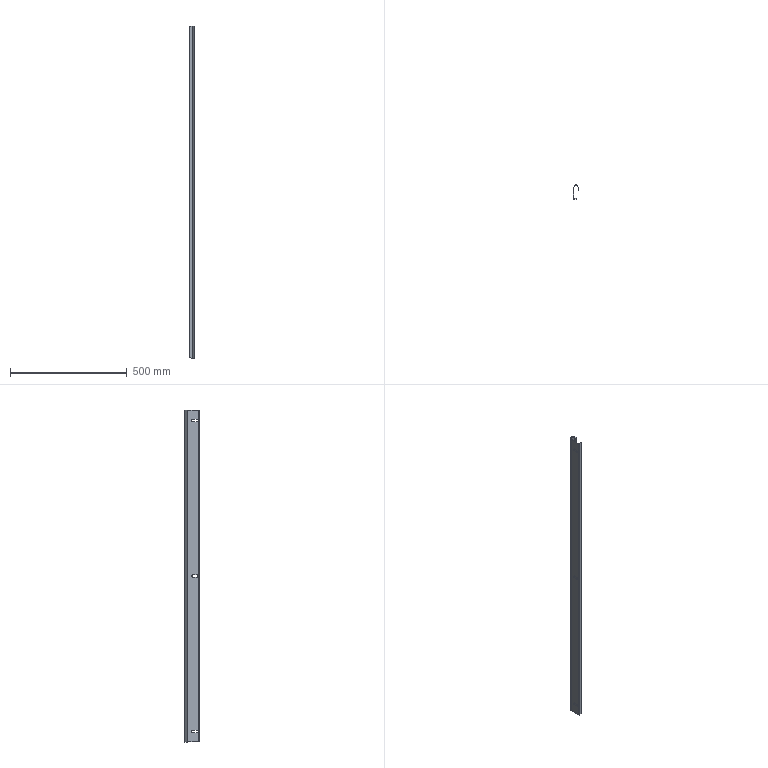Part | STEP file | Sliding Door Lower Rail | 1 solid | 34 faces | box 24 x 61.13 x 1420 mm | volume 280395 mm3 | plane 20 | cylinder 14 | commonest cylinder face diameters 9 x6 0.2 x4 4.2 x4
STEP:
#1=CARTESIAN_POINT('',(-22.,-489.271,1420.));
#2=VERTEX_POINT('',#1);
#3=CARTESIAN_POINT('',(-22.,-442.241,1420.));
#4=VERTEX_POINT('',#3);
#5=CARTESIAN_POINT('',(-22.,-441.371,1420.));
#6=DIRECTION('',(0.,1.,0.));
#7=VECTOR('',#6,1000.);
#8=LINE('',#5,#7);
#9=EDGE_CURVE('',#2,#4,#8,.T.);
#10=ORIENTED_EDGE('',*,*,#9,.T.);
#11=CARTESIAN_POINT('',(-22.,-442.241,0.));
#12=VERTEX_POINT('',#11);
#13=CARTESIAN_POINT('',(-22.,-442.241,1420.));
#14=DIRECTION('',(0.,0.,-1.));
#15=VECTOR('',#14,1000.);
#16=LINE('',#13,#15);
#17=EDGE_CURVE('',#4,#12,#16,.T.);
#18=ORIENTED_EDGE('',*,*,#17,.T.);
#19=CARTESIAN_POINT('',(-22.,-489.271,0.));
#20=VERTEX_POINT('',#19);
#21=CARTESIAN_POINT('',(-22.,-441.371,0.));
#22=DIRECTION('',(0.,-1.,0.));
#23=VECTOR('',#22,1000.);
#24=LINE('',#21,#23);
#25=EDGE_CURVE('',#12,#20,#24,.T.);
#26=ORIENTED_EDGE('',*,*,#25,.T.);
#27=CARTESIAN_POINT('',(-22.,-489.271,1420.));
#28=DIRECTION('',(0.,0.,1.));
#29=VECTOR('',#28,1000.);
#30=LINE('',#27,#29);
#31=EDGE_CURVE('',#20,#2,#30,.T.);
#32=ORIENTED_EDGE('',*,*,#31,.T.);
#33=EDGE_LOOP('',(#10,#18,#26,#32));
#34=FACE_OUTER_BOUND('',#33,.T.);
#35=CARTESIAN_POINT('',(-22.,-483.371,1379.5));
#36=VERTEX_POINT('',#35);
#37=CARTESIAN_POINT('',(-22.,-483.371,1370.5));
#38=VERTEX_POINT('',#37);
#39=CARTESIAN_POINT('',(-22.,-483.371,1375.));
#40=DIRECTION('',(1.,0.,0.));
#41=DIRECTION('',(0.,0.,-1.));
#42=AXIS2_PLACEMENT_3D('',#39,#40,#41);
#43=CIRCLE('',#42,4.5);
#44=EDGE_CURVE('',#36,#38,#43,.T.);
#45=ORIENTED_EDGE('',*,*,#44,.T.);
#46=CARTESIAN_POINT('',(-22.,-463.371,1370.5));
#47=VERTEX_POINT('',#46);
#48=CARTESIAN_POINT('',(-22.,-441.371,1370.5));
#49=DIRECTION('',(0.,1.,0.));
#50=VECTOR('',#49,1000.);
#51=LINE('',#48,#50);
#52=EDGE_CURVE('',#38,#47,#51,.T.);
#53=ORIENTED_EDGE('',*,*,#52,.T.);
#54=CARTESIAN_POINT('',(-22.,-463.371,1379.5));
#55=VERTEX_POINT('',#54);
#56=CARTESIAN_POINT('',(-22.,-463.371,1375.));
#57=DIRECTION('',(1.,0.,0.));
#58=DIRECTION('',(0.,0.,-1.));
#59=AXIS2_PLACEMENT_3D('',#56,#57,#58);
#60=CIRCLE('',#59,4.5);
#61=EDGE_CURVE('',#47,#55,#60,.T.);
#62=ORIENTED_EDGE('',*,*,#61,.T.);
#63=CARTESIAN_POINT('',(-22.,-441.371,1379.5));
#64=DIRECTION('',(0.,-1.,0.));
#65=VECTOR('',#64,1000.);
#66=LINE('',#63,#65);
#67=EDGE_CURVE('',#55,#36,#66,.T.);
#68=ORIENTED_EDGE('',*,*,#67,.T.);
#69=EDGE_LOOP('',(#45,#53,#62,#68));
#70=FACE_BOUND('',#69,.T.);
#71=CARTESIAN_POINT('',(-22.,-483.371,714.5));
#72=VERTEX_POINT('',#71);
#73=CARTESIAN_POINT('',(-22.,-483.371,705.5));
#74=VERTEX_POINT('',#73);
#75=CARTESIAN_POINT('',(-22.,-483.371,710.));
#76=DIRECTION('',(1.,0.,0.));
#77=DIRECTION('',(0.,0.,-1.));
#78=AXIS2_PLACEMENT_3D('',#75,#76,#77);
#79=CIRCLE('',#78,4.5);
#80=EDGE_CURVE('',#72,#74,#79,.T.);
#81=ORIENTED_EDGE('',*,*,#80,.T.);
#82=CARTESIAN_POINT('',(-22.,-463.371,705.5));
#83=VERTEX_POINT('',#82);
#84=CARTESIAN_POINT('',(-22.,-441.371,705.5));
#85=DIRECTION('',(0.,1.,0.));
#86=VECTOR('',#85,1000.);
#87=LINE('',#84,#86);
#88=EDGE_CURVE('',#74,#83,#87,.T.);
#89=ORIENTED_EDGE('',*,*,#88,.T.);
#90=CARTESIAN_POINT('',(-22.,-463.371,714.5));
#91=VERTEX_POINT('',#90);
#92=CARTESIAN_POINT('',(-22.,-463.371,710.));
#93=DIRECTION('',(1.,0.,0.));
#94=DIRECTION('',(0.,0.,-1.));
#95=AXIS2_PLACEMENT_3D('',#92,#93,#94);
#96=CIRCLE('',#95,4.5);
#97=EDGE_CURVE('',#83,#91,#96,.T.);
#98=ORIENTED_EDGE('',*,*,#97,.T.);
#99=CARTESIAN_POINT('',(-22.,-441.371,714.5));
#100=DIRECTION('',(0.,-1.,0.));
#101=VECTOR('',#100,1000.);
#102=LINE('',#99,#101);
#103=EDGE_CURVE('',#91,#72,#102,.T.);
#104=ORIENTED_EDGE('',*,*,#103,.T.);
#105=EDGE_LOOP('',(#81,#89,#98,#104));
#106=FACE_BOUND('',#105,.T.);
#107=CARTESIAN_POINT('',(-22.,-483.371,49.5));
#108=VERTEX_POINT('',#107);
#109=CARTESIAN_POINT('',(-22.,-483.371,40.5));
#110=VERTEX_POINT('',#109);
#111=CARTESIAN_POINT('',(-22.,-483.371,45.));
#112=DIRECTION('',(1.,0.,0.));
#113=DIRECTION('',(0.,0.,-1.));
#114=AXIS2_PLACEMENT_3D('',#111,#112,#113);
#115=CIRCLE('',#114,4.5);
#116=EDGE_CURVE('',#108,#110,#115,.T.);
#117=ORIENTED_EDGE('',*,*,#116,.T.);
#118=CARTESIAN_POINT('',(-22.,-463.371,40.5));
#119=VERTEX_POINT('',#118);
#120=CARTESIAN_POINT('',(-22.,-441.371,40.5));
#121=DIRECTION('',(0.,1.,0.));
#122=VECTOR('',#121,1000.);
#123=LINE('',#120,#122);
#124=EDGE_CURVE('',#110,#119,#123,.T.);
#125=ORIENTED_EDGE('',*,*,#124,.T.);
#126=CARTESIAN_POINT('',(-22.,-463.371,49.5));
#127=VERTEX_POINT('',#126);
#128=CARTESIAN_POINT('',(-22.,-463.371,45.));
#129=DIRECTION('',(1.,0.,0.));
#130=DIRECTION('',(0.,0.,-1.));
#131=AXIS2_PLACEMENT_3D('',#128,#129,#130);
#132=CIRCLE('',#131,4.5);
#133=EDGE_CURVE('',#119,#127,#132,.T.);
#134=ORIENTED_EDGE('',*,*,#133,.T.);
#135=CARTESIAN_POINT('',(-22.,-441.371,49.5));
#136=DIRECTION('',(0.,-1.,0.));
#137=VECTOR('',#136,1000.);
#138=LINE('',#135,#137);
#139=EDGE_CURVE('',#127,#108,#138,.T.);
#140=ORIENTED_EDGE('',*,*,#139,.T.);
#141=EDGE_LOOP('',(#117,#125,#134,#140));
#142=FACE_BOUND('',#141,.T.);
#143=CARTESIAN_POINT('',(-22.,-441.371,1420.));
#144=DIRECTION('',(-1.,0.,0.));
#145=DIRECTION('',(0.,-1.,0.));
#146=AXIS2_PLACEMENT_3D('',#143,#144,#145);
#147=PLANE('',#146);
#148=ADVANCED_FACE('',(#34,#70,#106,#142),#147,.T.);
#149=CARTESIAN_POINT('',(-21.385,-440.756,1420.));
#150=VERTEX_POINT('',#149);
#151=CARTESIAN_POINT('',(-19.9,-442.241,1420.));
#152=DIRECTION('',(0.,0.,1.));
#153=DIRECTION('',(-1.,0.,0.));
#154=AXIS2_PLACEMENT_3D('',#151,#152,#153);
#155=CIRCLE('',#154,2.1);
#156=EDGE_CURVE('',#150,#4,#155,.T.);
#157=ORIENTED_EDGE('',*,*,#156,.F.);
#158=CARTESIAN_POINT('',(-21.385,-440.756,0.));
#159=VERTEX_POINT('',#158);
#160=CARTESIAN_POINT('',(-21.385,-440.756,1420.));
#161=DIRECTION('',(0.,0.,-1.));
#162=VECTOR('',#161,1000.);
#163=LINE('',#160,#162);
#164=EDGE_CURVE('',#150,#159,#163,.T.);
#165=ORIENTED_EDGE('',*,*,#164,.T.);
#166=CARTESIAN_POINT('',(-19.9,-442.241,0.));
#167=DIRECTION('',(0.,0.,-1.));
#168=DIRECTION('',(-1.,0.,0.));
#169=AXIS2_PLACEMENT_3D('',#166,#167,#168);
#170=CIRCLE('',#169,2.1);
#171=EDGE_CURVE('',#12,#159,#170,.T.);
#172=ORIENTED_EDGE('',*,*,#171,.F.);
#173=ORIENTED_EDGE('',*,*,#17,.F.);
#174=EDGE_LOOP('',(#157,#165,#172,#173));
#175=FACE_OUTER_BOUND('',#174,.T.);
#176=CARTESIAN_POINT('',(-19.9,-442.241,1420.));
#177=DIRECTION('',(0.,0.,-1.));
#178=DIRECTION('',(-1.,0.,0.));
#179=AXIS2_PLACEMENT_3D('',#176,#177,#178);
#180=CYLINDRICAL_SURFACE('',#179,2.1);
#181=ADVANCED_FACE('',(#175),#180,.T.);
#182=CARTESIAN_POINT('',(-20.,-489.271,1420.));
#183=VERTEX_POINT('',#182);
#184=CARTESIAN_POINT('',(-20.,-442.241,1420.));
#185=VERTEX_POINT('',#184);
#186=CARTESIAN_POINT('',(-20.,-489.371,1420.));
#187=DIRECTION('',(0.,1.,0.));
#188=VECTOR('',#187,1000.);
#189=LINE('',#186,#188);
#190=EDGE_CURVE('',#183,#185,#189,.T.);
#191=ORIENTED_EDGE('',*,*,#190,.T.);
#192=CARTESIAN_POINT('',(-19.971,-442.171,1420.));
#193=VERTEX_POINT('',#192);
#194=CARTESIAN_POINT('',(-19.9,-442.241,1420.));
#195=DIRECTION('',(0.,0.,-1.));
#196=DIRECTION('',(-1.,0.,0.));
#197=AXIS2_PLACEMENT_3D('',#194,#195,#196);
#198=CIRCLE('',#197,0.1);
#199=EDGE_CURVE('',#185,#193,#198,.T.);
#200=ORIENTED_EDGE('',*,*,#199,.T.);
#201=CARTESIAN_POINT('',(-10.071,-432.271,1420.));
#202=VERTEX_POINT('',#201);
#203=CARTESIAN_POINT('',(-19.971,-442.171,1420.));
#204=DIRECTION('',(0.7071,0.7071,0.));
#205=VECTOR('',#204,1000.);
#206=LINE('',#203,#205);
#207=EDGE_CURVE('',#193,#202,#206,.T.);
#208=ORIENTED_EDGE('',*,*,#207,.T.);
#209=CARTESIAN_POINT('',(-9.929,-432.271,1420.));
#210=VERTEX_POINT('',#209);
#211=CARTESIAN_POINT('',(-10.,-432.341,1420.));
#212=DIRECTION('',(0.,0.,-1.));
#213=DIRECTION('',(-1.,0.,0.));
#214=AXIS2_PLACEMENT_3D('',#211,#212,#213);
#215=CIRCLE('',#214,0.1);
#216=EDGE_CURVE('',#202,#210,#215,.T.);
#217=ORIENTED_EDGE('',*,*,#216,.T.);
#218=CARTESIAN_POINT('',(-0.02929,-442.171,1420.));
#219=VERTEX_POINT('',#218);
#220=CARTESIAN_POINT('',(-9.929,-432.271,1420.));
#221=DIRECTION('',(0.7071,-0.7071,0.));
#222=VECTOR('',#221,1000.);
#223=LINE('',#220,#222);
#224=EDGE_CURVE('',#210,#219,#223,.T.);
#225=ORIENTED_EDGE('',*,*,#224,.T.);
#226=CARTESIAN_POINT('',(0.000000001,-442.241,1420.));
#227=VERTEX_POINT('',#226);
#228=CARTESIAN_POINT('',(-0.1,-442.241,1420.));
#229=DIRECTION('',(0.,0.,-1.));
#230=DIRECTION('',(-1.,0.,0.));
#231=AXIS2_PLACEMENT_3D('',#228,#229,#230);
#232=CIRCLE('',#231,0.1);
#233=EDGE_CURVE('',#219,#227,#232,.T.);
#234=ORIENTED_EDGE('',*,*,#233,.T.);
#235=CARTESIAN_POINT('',(0.000000001,-451.371,1420.));
#236=VERTEX_POINT('',#235);
#237=CARTESIAN_POINT('',(0.000000001,-442.171,1420.));
#238=DIRECTION('',(0.,-1.,0.));
#239=VECTOR('',#238,1000.);
#240=LINE('',#237,#239);
#241=EDGE_CURVE('',#227,#236,#240,.T.);
#242=ORIENTED_EDGE('',*,*,#241,.T.);
#243=CARTESIAN_POINT('',(2.,-451.371,1420.));
#244=VERTEX_POINT('',#243);
#245=CARTESIAN_POINT('',(2.,-451.371,1420.));
#246=DIRECTION('',(-1.,0.,0.));
#247=VECTOR('',#246,1000.);
#248=LINE('',#245,#247);
#249=EDGE_CURVE('',#244,#236,#248,.T.);
#250=ORIENTED_EDGE('',*,*,#249,.F.);
#251=CARTESIAN_POINT('',(2.,-442.241,1420.));
#252=VERTEX_POINT('',#251);
#253=CARTESIAN_POINT('',(2.,-441.371,1420.));
#254=DIRECTION('',(0.,-1.,0.));
#255=VECTOR('',#254,1000.);
#256=LINE('',#253,#255);
#257=EDGE_CURVE('',#252,#244,#256,.T.);
#258=ORIENTED_EDGE('',*,*,#257,.F.);
#259=CARTESIAN_POINT('',(1.385,-440.756,1420.));
#260=VERTEX_POINT('',#259);
#261=CARTESIAN_POINT('',(-0.1,-442.241,1420.));
#262=DIRECTION('',(0.,0.,1.));
#263=DIRECTION('',(-1.,0.,0.));
#264=AXIS2_PLACEMENT_3D('',#261,#262,#263);
#265=CIRCLE('',#264,2.1);
#266=EDGE_CURVE('',#252,#260,#265,.T.);
#267=ORIENTED_EDGE('',*,*,#266,.T.);
#268=CARTESIAN_POINT('',(-8.515,-430.856,1420.));
#269=VERTEX_POINT('',#268);
#270=CARTESIAN_POINT('',(-10.,-429.371,1420.));
#271=DIRECTION('',(0.7071,-0.7071,0.));
#272=VECTOR('',#271,1000.);
#273=LINE('',#270,#272);
#274=EDGE_CURVE('',#269,#260,#273,.T.);
#275=ORIENTED_EDGE('',*,*,#274,.F.);
#276=CARTESIAN_POINT('',(-11.485,-430.856,1420.));
#277=VERTEX_POINT('',#276);
#278=CARTESIAN_POINT('',(-10.,-432.341,1420.));
#279=DIRECTION('',(0.,0.,-1.));
#280=DIRECTION('',(-1.,0.,0.));
#281=AXIS2_PLACEMENT_3D('',#278,#279,#280);
#282=CIRCLE('',#281,2.1);
#283=EDGE_CURVE('',#277,#269,#282,.T.);
#284=ORIENTED_EDGE('',*,*,#283,.F.);
#285=CARTESIAN_POINT('',(-22.,-441.371,1420.));
#286=DIRECTION('',(0.7071,0.7071,0.));
#287=VECTOR('',#286,1000.);
#288=LINE('',#285,#287);
#289=EDGE_CURVE('',#150,#277,#288,.T.);
#290=ORIENTED_EDGE('',*,*,#289,.F.);
#291=ORIENTED_EDGE('',*,*,#156,.T.);
#292=ORIENTED_EDGE('',*,*,#9,.F.);
#293=CARTESIAN_POINT('',(-19.9,-491.371,1420.));
#294=VERTEX_POINT('',#293);
#295=CARTESIAN_POINT('',(-19.9,-489.271,1420.));
#296=DIRECTION('',(0.,0.,-1.));
#297=DIRECTION('',(-1.,0.,0.));
#298=AXIS2_PLACEMENT_3D('',#295,#296,#297);
#299=CIRCLE('',#298,2.1);
#300=EDGE_CURVE('',#294,#2,#299,.T.);
#301=ORIENTED_EDGE('',*,*,#300,.F.);
#302=CARTESIAN_POINT('',(-10.,-491.371,1420.));
#303=VERTEX_POINT('',#302);
#304=CARTESIAN_POINT('',(-22.,-491.371,1420.));
#305=DIRECTION('',(-1.,0.,0.));
#306=VECTOR('',#305,1000.);
#307=LINE('',#304,#306);
#308=EDGE_CURVE('',#303,#294,#307,.T.);
#309=ORIENTED_EDGE('',*,*,#308,.F.);
#310=CARTESIAN_POINT('',(-10.,-489.371,1420.));
#311=VERTEX_POINT('',#310);
#312=CARTESIAN_POINT('',(-10.,-442.241,1420.));
#313=DIRECTION('',(0.,1.,0.));
#314=VECTOR('',#313,1000.);
#315=LINE('',#312,#314);
#316=EDGE_CURVE('',#303,#311,#315,.T.);
#317=ORIENTED_EDGE('',*,*,#316,.T.);
#318=CARTESIAN_POINT('',(-19.9,-489.371,1420.));
#319=VERTEX_POINT('',#318);
#320=CARTESIAN_POINT('',(-0.1,-489.371,1420.));
#321=DIRECTION('',(-1.,0.,0.));
#322=VECTOR('',#321,1000.);
#323=LINE('',#320,#322);
#324=EDGE_CURVE('',#311,#319,#323,.T.);
#325=ORIENTED_EDGE('',*,*,#324,.T.);
#326=CARTESIAN_POINT('',(-19.9,-489.271,1420.));
#327=DIRECTION('',(0.,0.,-1.));
#328=DIRECTION('',(-1.,0.,0.));
#329=AXIS2_PLACEMENT_3D('',#326,#327,#328);
#330=CIRCLE('',#329,0.1);
#331=EDGE_CURVE('',#319,#183,#330,.T.);
#332=ORIENTED_EDGE('',*,*,#331,.T.);
#333=EDGE_LOOP('',(#191,#200,#208,#217,#225,#234,#242,#250,#258,#267,#275,#284,#290,#291,#292,#301,#309,#317,#325,#332));
#334=FACE_OUTER_BOUND('',#333,.T.);
#335=CARTESIAN_POINT('',(-19.9,-489.371,1420.));
#336=DIRECTION('',(0.,0.,1.));
#337=DIRECTION('',(1.,0.,0.));
#338=AXIS2_PLACEMENT_3D('',#335,#336,#337);
#339=PLANE('',#338);
#340=ADVANCED_FACE('',(#334),#339,.T.);
#341=ORIENTED_EDGE('',*,*,#300,.T.);
#342=ORIENTED_EDGE('',*,*,#31,.F.);
#343=CARTESIAN_POINT('',(-19.9,-491.371,0.));
#344=VERTEX_POINT('',#343);
#345=CARTESIAN_POINT('',(-19.9,-489.271,0.));
#346=DIRECTION('',(0.,0.,1.));
#347=DIRECTION('',(-1.,0.,0.));
#348=AXIS2_PLACEMENT_3D('',#345,#346,#347);
#349=CIRCLE('',#348,2.1);
#350=EDGE_CURVE('',#20,#344,#349,.T.);
#351=ORIENTED_EDGE('',*,*,#350,.T.);
#352=CARTESIAN_POINT('',(-19.9,-491.371,1420.));
#353=DIRECTION('',(0.,0.,1.));
#354=VECTOR('',#353,1000.);
#355=LINE('',#352,#354);
#356=EDGE_CURVE('',#344,#294,#355,.T.);
#357=ORIENTED_EDGE('',*,*,#356,.T.);
#358=EDGE_LOOP('',(#341,#342,#351,#357));
#359=FACE_OUTER_BOUND('',#358,.T.);
#360=CARTESIAN_POINT('',(-19.9,-489.271,1420.));
#361=DIRECTION('',(0.,0.,-1.));
#362=DIRECTION('',(-1.,0.,0.));
#363=AXIS2_PLACEMENT_3D('',#360,#361,#362);
#364=CYLINDRICAL_SURFACE('',#363,2.1);
#365=ADVANCED_FACE('',(#359),#364,.T.);
#366=CARTESIAN_POINT('',(-20.,-442.241,0.));
#367=VERTEX_POINT('',#366);
#368=CARTESIAN_POINT('',(-20.,-489.271,0.));
#369=VERTEX_POINT('',#368);
#370=CARTESIAN_POINT('',(-20.,-442.171,0.));
#371=DIRECTION('',(0.,-1.,0.));
#372=VECTOR('',#371,1000.);
#373=LINE('',#370,#372);
#374=EDGE_CURVE('',#367,#369,#373,.T.);
#375=ORIENTED_EDGE('',*,*,#374,.T.);
#376=CARTESIAN_POINT('',(-19.9,-489.371,0.));
#377=VERTEX_POINT('',#376);
#378=CARTESIAN_POINT('',(-19.9,-489.271,0.));
#379=DIRECTION('',(0.,0.,1.));
#380=DIRECTION('',(-1.,0.,0.));
#381=AXIS2_PLACEMENT_3D('',#378,#379,#380);
#382=CIRCLE('',#381,0.1);
#383=EDGE_CURVE('',#369,#377,#382,.T.);
#384=ORIENTED_EDGE('',*,*,#383,.T.);
#385=CARTESIAN_POINT('',(-10.,-489.371,0.));
#386=VERTEX_POINT('',#385);
#387=CARTESIAN_POINT('',(-20.,-489.371,0.));
#388=DIRECTION('',(1.,0.,0.));
#389=VECTOR('',#388,1000.);
#390=LINE('',#387,#389);
#391=EDGE_CURVE('',#377,#386,#390,.T.);
#392=ORIENTED_EDGE('',*,*,#391,.T.);
#393=CARTESIAN_POINT('',(-10.,-491.371,0.));
#394=VERTEX_POINT('',#393);
#395=CARTESIAN_POINT('',(-10.,-489.371,0.));
#396=DIRECTION('',(0.,1.,0.));
#397=VECTOR('',#396,1000.);
#398=LINE('',#395,#397);
#399=EDGE_CURVE('',#394,#386,#398,.T.);
#400=ORIENTED_EDGE('',*,*,#399,.F.);
#401=CARTESIAN_POINT('',(-22.,-491.371,0.));
#402=DIRECTION('',(1.,0.,0.));
#403=VECTOR('',#402,1000.);
#404=LINE('',#401,#403);
#405=EDGE_CURVE('',#344,#394,#404,.T.);
#406=ORIENTED_EDGE('',*,*,#405,.F.);
#407=ORIENTED_EDGE('',*,*,#350,.F.);
#408=ORIENTED_EDGE('',*,*,#25,.F.);
#409=ORIENTED_EDGE('',*,*,#171,.T.);
#410=CARTESIAN_POINT('',(-11.485,-430.856,0.));
#411=VERTEX_POINT('',#410);
#412=CARTESIAN_POINT('',(-22.,-441.371,0.));
#413=DIRECTION('',(-0.7071,-0.7071,0.));
#414=VECTOR('',#413,1000.);
#415=LINE('',#412,#414);
#416=EDGE_CURVE('',#411,#159,#415,.T.);
#417=ORIENTED_EDGE('',*,*,#416,.F.);
#418=CARTESIAN_POINT('',(-8.515,-430.856,0.));
#419=VERTEX_POINT('',#418);
#420=CARTESIAN_POINT('',(-10.,-432.341,0.));
#421=DIRECTION('',(0.,0.,1.));
#422=DIRECTION('',(-1.,0.,0.));
#423=AXIS2_PLACEMENT_3D('',#420,#421,#422);
#424=CIRCLE('',#423,2.1);
#425=EDGE_CURVE('',#419,#411,#424,.T.);
#426=ORIENTED_EDGE('',*,*,#425,.F.);
#427=CARTESIAN_POINT('',(1.385,-440.756,0.));
#428=VERTEX_POINT('',#427);
#429=CARTESIAN_POINT('',(-10.,-429.371,0.));
#430=DIRECTION('',(-0.7071,0.7071,0.));
#431=VECTOR('',#430,1000.);
#432=LINE('',#429,#431);
#433=EDGE_CURVE('',#428,#419,#432,.T.);
#434=ORIENTED_EDGE('',*,*,#433,.F.);
#435=CARTESIAN_POINT('',(2.,-442.241,0.));
#436=VERTEX_POINT('',#435);
#437=CARTESIAN_POINT('',(-0.1,-442.241,0.));
#438=DIRECTION('',(0.,0.,-1.));
#439=DIRECTION('',(-1.,0.,0.));
#440=AXIS2_PLACEMENT_3D('',#437,#438,#439);
#441=CIRCLE('',#440,2.1);
#442=EDGE_CURVE('',#428,#436,#441,.T.);
#443=ORIENTED_EDGE('',*,*,#442,.T.);
#444=CARTESIAN_POINT('',(2.,-451.371,0.));
#445=VERTEX_POINT('',#444);
#446=CARTESIAN_POINT('',(2.,-441.371,0.));
#447=DIRECTION('',(0.,1.,0.));
#448=VECTOR('',#447,1000.);
#449=LINE('',#446,#448);
#450=EDGE_CURVE('',#445,#436,#449,.T.);
#451=ORIENTED_EDGE('',*,*,#450,.F.);
#452=CARTESIAN_POINT('',(0.000000001,-451.371,0.));
#453=VERTEX_POINT('',#452);
#454=CARTESIAN_POINT('',(2.,-451.371,0.));
#455=DIRECTION('',(1.,0.,0.));
#456=VECTOR('',#455,1000.);
#457=LINE('',#454,#456);
#458=EDGE_CURVE('',#453,#445,#457,.T.);
#459=ORIENTED_EDGE('',*,*,#458,.F.);
#460=CARTESIAN_POINT('',(0.000000001,-442.241,0.));
#461=VERTEX_POINT('',#460);
#462=CARTESIAN_POINT('',(0.000000001,-442.241,0.));
#463=DIRECTION('',(0.,-1.,0.));
#464=VECTOR('',#463,1000.);
#465=LINE('',#462,#464);
#466=EDGE_CURVE('',#461,#453,#465,.T.);
#467=ORIENTED_EDGE('',*,*,#466,.F.);
#468=CARTESIAN_POINT('',(-0.02929,-442.171,0.));
#469=VERTEX_POINT('',#468);
#470=CARTESIAN_POINT('',(-0.1,-442.241,0.));
#471=DIRECTION('',(0.,0.,1.));
#472=DIRECTION('',(-1.,0.,0.));
#473=AXIS2_PLACEMENT_3D('',#470,#471,#472);
#474=CIRCLE('',#473,0.1);
#475=EDGE_CURVE('',#461,#469,#474,.T.);
#476=ORIENTED_EDGE('',*,*,#475,.T.);
#477=CARTESIAN_POINT('',(-9.929,-432.271,0.));
#478=VERTEX_POINT('',#477);
#479=CARTESIAN_POINT('',(-0.02929,-442.171,0.));
#480=DIRECTION('',(-0.7071,0.7071,0.));
#481=VECTOR('',#480,1000.);
#482=LINE('',#479,#481);
#483=EDGE_CURVE('',#469,#478,#482,.T.);
#484=ORIENTED_EDGE('',*,*,#483,.T.);
#485=CARTESIAN_POINT('',(-10.071,-432.271,0.));
#486=VERTEX_POINT('',#485);
#487=CARTESIAN_POINT('',(-10.,-432.341,0.));
#488=DIRECTION('',(0.,0.,1.));
#489=DIRECTION('',(-1.,0.,0.));
#490=AXIS2_PLACEMENT_3D('',#487,#488,#489);
#491=CIRCLE('',#490,0.1);
#492=EDGE_CURVE('',#478,#486,#491,.T.);
#493=ORIENTED_EDGE('',*,*,#492,.T.);
#494=CARTESIAN_POINT('',(-19.971,-442.171,0.));
#495=VERTEX_POINT('',#494);
#496=CARTESIAN_POINT('',(-10.071,-432.271,0.));
#497=DIRECTION('',(-0.7071,-0.7071,0.));
#498=VECTOR('',#497,1000.);
#499=LINE('',#496,#498);
#500=EDGE_CURVE('',#486,#495,#499,.T.);
#501=ORIENTED_EDGE('',*,*,#500,.T.);
#502=CARTESIAN_POINT('',(-19.9,-442.241,0.));
#503=DIRECTION('',(0.,0.,1.));
#504=DIRECTION('',(-1.,0.,0.));
#505=AXIS2_PLACEMENT_3D('',#502,#503,#504);
#506=CIRCLE('',#505,0.1);
#507=EDGE_CURVE('',#495,#367,#506,.T.);
#508=ORIENTED_EDGE('',*,*,#507,.T.);
#509=EDGE_LOOP('',(#375,#384,#392,#400,#406,#407,#408,#409,#417,#426,#434,#443,#451,#459,#467,#476,#484,#493,#501,#508));
#510=FACE_OUTER_BOUND('',#509,.T.);
#511=CARTESIAN_POINT('',(-19.971,-442.171,0.));
#512=DIRECTION('',(0.,0.,-1.));
#513=DIRECTION('',(-1.,0.,0.));
#514=AXIS2_PLACEMENT_3D('',#511,#512,#513);
#515=PLANE('',#514);
#516=ADVANCED_FACE('',(#510),#515,.T.);
#517=CARTESIAN_POINT('',(-20.,-483.371,1370.5));
#518=VERTEX_POINT('',#517);
#519=CARTESIAN_POINT('',(-30.,-483.371,1370.5));
#520=DIRECTION('',(-1.,0.,0.));
#521=VECTOR('',#520,1000.);
#522=LINE('',#519,#521);
#523=EDGE_CURVE('',#518,#38,#522,.T.);
#524=ORIENTED_EDGE('',*,*,#523,.F.);
#525=CARTESIAN_POINT('',(-20.,-463.371,1370.5));
#526=VERTEX_POINT('',#525);
#527=CARTESIAN_POINT('',(-20.,-463.371,1370.5));
#528=DIRECTION('',(0.,-1.,0.));
#529=VECTOR('',#528,1000.);
#530=LINE('',#527,#529);
#531=EDGE_CURVE('',#526,#518,#530,.T.);
#532=ORIENTED_EDGE('',*,*,#531,.F.);
#533=CARTESIAN_POINT('',(-30.,-463.371,1370.5));
#534=DIRECTION('',(1.,0.,0.));
#535=VECTOR('',#534,1000.);
#536=LINE('',#533,#535);
#537=EDGE_CURVE('',#47,#526,#536,.T.);
#538=ORIENTED_EDGE('',*,*,#537,.F.);
#539=ORIENTED_EDGE('',*,*,#52,.F.);
#540=EDGE_LOOP('',(#524,#532,#538,#539));
#541=FACE_OUTER_BOUND('',#540,.T.);
#542=CARTESIAN_POINT('',(-30.,-463.371,1370.5));
#543=DIRECTION('',(0.,0.,-1.));
#544=DIRECTION('',(-1.,0.,0.));
#545=AXIS2_PLACEMENT_3D('',#542,#543,#544);
#546=PLANE('',#545);
#547=ADVANCED_FACE('',(#541),#546,.F.);
#548=CARTESIAN_POINT('',(-20.,-483.371,1379.5));
#549=VERTEX_POINT('',#548);
#550=CARTESIAN_POINT('',(-30.,-483.371,1379.5));
#551=DIRECTION('',(-1.,0.,0.));
#552=VECTOR('',#551,1000.);
#553=LINE('',#550,#552);
#554=EDGE_CURVE('',#549,#36,#553,.T.);
#555=ORIENTED_EDGE('',*,*,#554,.F.);
#556=CARTESIAN_POINT('',(-20.,-483.371,1375.));
#557=DIRECTION('',(-1.,0.,0.));
#558=DIRECTION('',(0.,0.,-1.));
#559=AXIS2_PLACEMENT_3D('',#556,#557,#558);
#560=CIRCLE('',#559,4.5);
#561=EDGE_CURVE('',#518,#549,#560,.T.);
#562=ORIENTED_EDGE('',*,*,#561,.F.);
#563=ORIENTED_EDGE('',*,*,#523,.T.);
#564=ORIENTED_EDGE('',*,*,#44,.F.);
#565=EDGE_LOOP('',(#555,#562,#563,#564));
#566=FACE_OUTER_BOUND('',#565,.T.);
#567=CARTESIAN_POINT('',(-30.,-483.371,1375.));
#568=DIRECTION('',(1.,0.,0.));
#569=DIRECTION('',(0.,0.,-1.));
#570=AXIS2_PLACEMENT_3D('',#567,#568,#569);
#571=CYLINDRICAL_SURFACE('',#570,4.5);
#572=ADVANCED_FACE('',(#566),#571,.F.);
#573=CARTESIAN_POINT('',(-20.,-463.371,1379.5));
#574=VERTEX_POINT('',#573);
#575=CARTESIAN_POINT('',(-30.,-463.371,1379.5));
#576=DIRECTION('',(-1.,0.,0.));
#577=VECTOR('',#576,1000.);
#578=LINE('',#575,#577);
#579=EDGE_CURVE('',#574,#55,#578,.T.);
#580=ORIENTED_EDGE('',*,*,#579,.F.);
#581=CARTESIAN_POINT('',(-20.,-463.371,1379.5));
#582=DIRECTION('',(0.,1.,0.));
#583=VECTOR('',#582,1000.);
#584=LINE('',#581,#583);
#585=EDGE_CURVE('',#549,#574,#584,.T.);
#586=ORIENTED_EDGE('',*,*,#585,.F.);
#587=ORIENTED_EDGE('',*,*,#554,.T.);
#588=ORIENTED_EDGE('',*,*,#67,.F.);
#589=EDGE_LOOP('',(#580,#586,#587,#588));
#590=FACE_OUTER_BOUND('',#589,.T.);
#591=CARTESIAN_POINT('',(-30.,-463.371,1379.5));
#592=DIRECTION('',(0.,0.,1.));
#593=DIRECTION('',(1.,0.,0.));
#594=AXIS2_PLACEMENT_3D('',#591,#592,#593);
#595=PLANE('',#594);
#596=ADVANCED_FACE('',(#590),#595,.F.);
#597=ORIENTED_EDGE('',*,*,#537,.T.);
#598=CARTESIAN_POINT('',(-20.,-463.371,1375.));
#599=DIRECTION('',(-1.,0.,0.));
#600=DIRECTION('',(0.,0.,-1.));
#601=AXIS2_PLACEMENT_3D('',#598,#599,#600);
#602=CIRCLE('',#601,4.5);
#603=EDGE_CURVE('',#574,#526,#602,.T.);
#604=ORIENTED_EDGE('',*,*,#603,.F.);
#605=ORIENTED_EDGE('',*,*,#579,.T.);
#606=ORIENTED_EDGE('',*,*,#61,.F.);
#607=EDGE_LOOP('',(#597,#604,#605,#606));
#608=FACE_OUTER_BOUND('',#607,.T.);
#609=CARTESIAN_POINT('',(-30.,-463.371,1375.));
#610=DIRECTION('',(1.,0.,0.));
#611=DIRECTION('',(0.,0.,-1.));
#612=AXIS2_PLACEMENT_3D('',#609,#610,#611);
#613=CYLINDRICAL_SURFACE('',#612,4.5);
#614=ADVANCED_FACE('',(#608),#613,.F.);
#615=CARTESIAN_POINT('',(-20.,-483.371,705.5));
#616=VERTEX_POINT('',#615);
#617=CARTESIAN_POINT('',(-30.,-483.371,705.5));
#618=DIRECTION('',(-1.,0.,0.));
#619=VECTOR('',#618,1000.);
#620=LINE('',#617,#619);
#621=EDGE_CURVE('',#616,#74,#620,.T.);
#622=ORIENTED_EDGE('',*,*,#621,.F.);
#623=CARTESIAN_POINT('',(-20.,-463.371,705.5));
#624=VERTEX_POINT('',#623);
#625=CARTESIAN_POINT('',(-20.,-463.371,705.5));
#626=DIRECTION('',(0.,-1.,0.));
#627=VECTOR('',#626,1000.);
#628=LINE('',#625,#627);
#629=EDGE_CURVE('',#624,#616,#628,.T.);
#630=ORIENTED_EDGE('',*,*,#629,.F.);
#631=CARTESIAN_POINT('',(-30.,-463.371,705.5));
#632=DIRECTION('',(1.,0.,0.));
#633=VECTOR('',#632,1000.);
#634=LINE('',#631,#633);
#635=EDGE_CURVE('',#83,#624,#634,.T.);
#636=ORIENTED_EDGE('',*,*,#635,.F.);
#637=ORIENTED_EDGE('',*,*,#88,.F.);
#638=EDGE_LOOP('',(#622,#630,#636,#637));
#639=FACE_OUTER_BOUND('',#638,.T.);
#640=CARTESIAN_POINT('',(-30.,-463.371,705.5));
#641=DIRECTION('',(0.,0.,-1.));
#642=DIRECTION('',(-1.,0.,0.));
#643=AXIS2_PLACEMENT_3D('',#640,#641,#642);
#644=PLANE('',#643);
#645=ADVANCED_FACE('',(#639),#644,.F.);
#646=CARTESIAN_POINT('',(-20.,-483.371,714.5));
#647=VERTEX_POINT('',#646);
#648=CARTESIAN_POINT('',(-30.,-483.371,714.5));
#649=DIRECTION('',(-1.,0.,0.));
#650=VECTOR('',#649,1000.);
#651=LINE('',#648,#650);
#652=EDGE_CURVE('',#647,#72,#651,.T.);
#653=ORIENTED_EDGE('',*,*,#652,.F.);
#654=CARTESIAN_POINT('',(-20.,-483.371,710.));
#655=DIRECTION('',(-1.,0.,0.));
#656=DIRECTION('',(0.,0.,-1.));
#657=AXIS2_PLACEMENT_3D('',#654,#655,#656);
#658=CIRCLE('',#657,4.5);
#659=EDGE_CURVE('',#616,#647,#658,.T.);
#660=ORIENTED_EDGE('',*,*,#659,.F.);
#661=ORIENTED_EDGE('',*,*,#621,.T.);
#662=ORIENTED_EDGE('',*,*,#80,.F.);
#663=EDGE_LOOP('',(#653,#660,#661,#662));
#664=FACE_OUTER_BOUND('',#663,.T.);
#665=CARTESIAN_POINT('',(-30.,-483.371,710.));
#666=DIRECTION('',(1.,0.,0.));
#667=DIRECTION('',(0.,0.,-1.));
#668=AXIS2_PLACEMENT_3D('',#665,#666,#667);
#669=CYLINDRICAL_SURFACE('',#668,4.5);
#670=ADVANCED_FACE('',(#664),#669,.F.);
#671=CARTESIAN_POINT('',(-20.,-463.371,714.5));
#672=VERTEX_POINT('',#671);
#673=CARTESIAN_POINT('',(-30.,-463.371,714.5));
#674=DIRECTION('',(-1.,0.,0.));
#675=VECTOR('',#674,1000.);
#676=LINE('',#673,#675);
#677=EDGE_CURVE('',#672,#91,#676,.T.);
#678=ORIENTED_EDGE('',*,*,#677,.F.);
#679=CARTESIAN_POINT('',(-20.,-463.371,714.5));
#680=DIRECTION('',(0.,1.,0.));
#681=VECTOR('',#680,1000.);
#682=LINE('',#679,#681);
#683=EDGE_CURVE('',#647,#672,#682,.T.);
#684=ORIENTED_EDGE('',*,*,#683,.F.);
#685=ORIENTED_EDGE('',*,*,#652,.T.);
#686=ORIENTED_EDGE('',*,*,#103,.F.);
#687=EDGE_LOOP('',(#678,#684,#685,#686));
#688=FACE_OUTER_BOUND('',#687,.T.);
#689=CARTESIAN_POINT('',(-30.,-463.371,714.5));
#690=DIRECTION('',(0.,0.,1.));
#691=DIRECTION('',(1.,0.,0.));
#692=AXIS2_PLACEMENT_3D('',#689,#690,#691);
#693=PLANE('',#692);
#694=ADVANCED_FACE('',(#688),#693,.F.);
#695=ORIENTED_EDGE('',*,*,#635,.T.);
#696=CARTESIAN_POINT('',(-20.,-463.371,710.));
#697=DIRECTION('',(-1.,0.,0.));
#698=DIRECTION('',(0.,0.,-1.));
#699=AXIS2_PLACEMENT_3D('',#696,#697,#698);
#700=CIRCLE('',#699,4.5);
#701=EDGE_CURVE('',#672,#624,#700,.T.);
#702=ORIENTED_EDGE('',*,*,#701,.F.);
#703=ORIENTED_EDGE('',*,*,#677,.T.);
#704=ORIENTED_EDGE('',*,*,#97,.F.);
#705=EDGE_LOOP('',(#695,#702,#703,#704));
#706=FACE_OUTER_BOUND('',#705,.T.);
#707=CARTESIAN_POINT('',(-30.,-463.371,710.));
#708=DIRECTION('',(1.,0.,0.));
#709=DIRECTION('',(0.,0.,-1.));
#710=AXIS2_PLACEMENT_3D('',#707,#708,#709);
#711=CYLINDRICAL_SURFACE('',#710,4.5);
#712=ADVANCED_FACE('',(#706),#711,.F.);
#713=CARTESIAN_POINT('',(-20.,-483.371,40.5));
#714=VERTEX_POINT('',#713);
#715=CARTESIAN_POINT('',(-30.,-483.371,40.5));
#716=DIRECTION('',(-1.,0.,0.));
#717=VECTOR('',#716,1000.);
#718=LINE('',#715,#717);
#719=EDGE_CURVE('',#714,#110,#718,.T.);
#720=ORIENTED_EDGE('',*,*,#719,.F.);
#721=CARTESIAN_POINT('',(-20.,-463.371,40.5));
#722=VERTEX_POINT('',#721);
#723=CARTESIAN_POINT('',(-20.,-463.371,40.5));
#724=DIRECTION('',(0.,-1.,0.));
#725=VECTOR('',#724,1000.);
#726=LINE('',#723,#725);
#727=EDGE_CURVE('',#722,#714,#726,.T.);
#728=ORIENTED_EDGE('',*,*,#727,.F.);
#729=CARTESIAN_POINT('',(-30.,-463.371,40.5));
#730=DIRECTION('',(1.,0.,0.));
#731=VECTOR('',#730,1000.);
#732=LINE('',#729,#731);
#733=EDGE_CURVE('',#119,#722,#732,.T.);
#734=ORIENTED_EDGE('',*,*,#733,.F.);
#735=ORIENTED_EDGE('',*,*,#124,.F.);
#736=EDGE_LOOP('',(#720,#728,#734,#735));
#737=FACE_OUTER_BOUND('',#736,.T.);
#738=CARTESIAN_POINT('',(-30.,-463.371,40.5));
#739=DIRECTION('',(0.,0.,-1.));
#740=DIRECTION('',(-1.,0.,0.));
#741=AXIS2_PLACEMENT_3D('',#738,#739,#740);
#742=PLANE('',#741);
#743=ADVANCED_FACE('',(#737),#742,.F.);
#744=CARTESIAN_POINT('',(-20.,-483.371,49.5));
#745=VERTEX_POINT('',#744);
#746=CARTESIAN_POINT('',(-30.,-483.371,49.5));
#747=DIRECTION('',(-1.,0.,0.));
#748=VECTOR('',#747,1000.);
#749=LINE('',#746,#748);
#750=EDGE_CURVE('',#745,#108,#749,.T.);
#751=ORIENTED_EDGE('',*,*,#750,.F.);
#752=CARTESIAN_POINT('',(-20.,-483.371,45.));
#753=DIRECTION('',(-1.,0.,0.));
#754=DIRECTION('',(0.,0.,-1.));
#755=AXIS2_PLACEMENT_3D('',#752,#753,#754);
#756=CIRCLE('',#755,4.5);
#757=EDGE_CURVE('',#714,#745,#756,.T.);
#758=ORIENTED_EDGE('',*,*,#757,.F.);
#759=ORIENTED_EDGE('',*,*,#719,.T.);
#760=ORIENTED_EDGE('',*,*,#116,.F.);
#761=EDGE_LOOP('',(#751,#758,#759,#760));
#762=FACE_OUTER_BOUND('',#761,.T.);
#763=CARTESIAN_POINT('',(-30.,-483.371,45.));
#764=DIRECTION('',(1.,0.,0.));
#765=DIRECTION('',(0.,0.,-1.));
#766=AXIS2_PLACEMENT_3D('',#763,#764,#765);
#767=CYLINDRICAL_SURFACE('',#766,4.5);
#768=ADVANCED_FACE('',(#762),#767,.F.);
#769=CARTESIAN_POINT('',(-20.,-463.371,49.5));
#770=VERTEX_POINT('',#769);
#771=CARTESIAN_POINT('',(-30.,-463.371,49.5));
#772=DIRECTION('',(-1.,0.,0.));
#773=VECTOR('',#772,1000.);
#774=LINE('',#771,#773);
#775=EDGE_CURVE('',#770,#127,#774,.T.);
#776=ORIENTED_EDGE('',*,*,#775,.F.);
#777=CARTESIAN_POINT('',(-20.,-463.371,49.5));
#778=DIRECTION('',(0.,1.,0.));
#779=VECTOR('',#778,1000.);
#780=LINE('',#777,#779);
#781=EDGE_CURVE('',#745,#770,#780,.T.);
#782=ORIENTED_EDGE('',*,*,#781,.F.);
#783=ORIENTED_EDGE('',*,*,#750,.T.);
#784=ORIENTED_EDGE('',*,*,#139,.F.);
#785=EDGE_LOOP('',(#776,#782,#783,#784));
#786=FACE_OUTER_BOUND('',#785,.T.);
#787=CARTESIAN_POINT('',(-30.,-463.371,49.5));
#788=DIRECTION('',(0.,0.,1.));
#789=DIRECTION('',(0.,-1.,0.));
#790=AXIS2_PLACEMENT_3D('',#787,#788,#789);
#791=PLANE('',#790);
#792=ADVANCED_FACE('',(#786),#791,.F.);
#793=ORIENTED_EDGE('',*,*,#733,.T.);
#794=CARTESIAN_POINT('',(-20.,-463.371,45.));
#795=DIRECTION('',(-1.,0.,0.));
#796=DIRECTION('',(0.,0.,-1.));
#797=AXIS2_PLACEMENT_3D('',#794,#795,#796);
#798=CIRCLE('',#797,4.5);
#799=EDGE_CURVE('',#770,#722,#798,.T.);
#800=ORIENTED_EDGE('',*,*,#799,.F.);
#801=ORIENTED_EDGE('',*,*,#775,.T.);
#802=ORIENTED_EDGE('',*,*,#133,.F.);
#803=EDGE_LOOP('',(#793,#800,#801,#802));
#804=FACE_OUTER_BOUND('',#803,.T.);
#805=CARTESIAN_POINT('',(-30.,-463.371,45.));
#806=DIRECTION('',(1.,0.,0.));
#807=DIRECTION('',(0.,0.,-1.));
#808=AXIS2_PLACEMENT_3D('',#805,#806,#807);
#809=CYLINDRICAL_SURFACE('',#808,4.5);
#810=ADVANCED_FACE('',(#804),#809,.F.);
#811=ORIENTED_EDGE('',*,*,#289,.T.);
#812=CARTESIAN_POINT('',(-11.485,-430.856,1420.));
#813=DIRECTION('',(0.,0.,-1.));
#814=VECTOR('',#813,1000.);
#815=LINE('',#812,#814);
#816=EDGE_CURVE('',#277,#411,#815,.T.);
#817=ORIENTED_EDGE('',*,*,#816,.T.);
#818=ORIENTED_EDGE('',*,*,#416,.T.);
#819=ORIENTED_EDGE('',*,*,#164,.F.);
#820=EDGE_LOOP('',(#811,#817,#818,#819));
#821=FACE_OUTER_BOUND('',#820,.T.);
#822=CARTESIAN_POINT('',(-22.,-441.371,1420.));
#823=DIRECTION('',(-0.7071,0.7071,0.));
#824=DIRECTION('',(-0.7071,-0.7071,0.));
#825=AXIS2_PLACEMENT_3D('',#822,#823,#824);
#826=PLANE('',#825);
#827=ADVANCED_FACE('',(#821),#826,.T.);
#828=CARTESIAN_POINT('',(-20.,-442.241,1420.));
#829=DIRECTION('',(0.,0.,-1.));
#830=VECTOR('',#829,1000.);
#831=LINE('',#828,#830);
#832=EDGE_CURVE('',#185,#367,#831,.T.);
#833=ORIENTED_EDGE('',*,*,#832,.F.);
#834=ORIENTED_EDGE('',*,*,#190,.F.);
#835=CARTESIAN_POINT('',(-20.,-489.271,1420.));
#836=DIRECTION('',(0.,0.,1.));
#837=VECTOR('',#836,1000.);
#838=LINE('',#835,#837);
#839=EDGE_CURVE('',#369,#183,#838,.T.);
#840=ORIENTED_EDGE('',*,*,#839,.F.);
#841=ORIENTED_EDGE('',*,*,#374,.F.);
#842=EDGE_LOOP('',(#833,#834,#840,#841));
#843=FACE_OUTER_BOUND('',#842,.T.);
#844=ORIENTED_EDGE('',*,*,#603,.T.);
#845=ORIENTED_EDGE('',*,*,#531,.T.);
#846=ORIENTED_EDGE('',*,*,#561,.T.);
#847=ORIENTED_EDGE('',*,*,#585,.T.);
#848=EDGE_LOOP('',(#844,#845,#846,#847));
#849=FACE_BOUND('',#848,.T.);
#850=ORIENTED_EDGE('',*,*,#701,.T.);
#851=ORIENTED_EDGE('',*,*,#629,.T.);
#852=ORIENTED_EDGE('',*,*,#659,.T.);
#853=ORIENTED_EDGE('',*,*,#683,.T.);
#854=EDGE_LOOP('',(#850,#851,#852,#853));
#855=FACE_BOUND('',#854,.T.);
#856=ORIENTED_EDGE('',*,*,#799,.T.);
#857=ORIENTED_EDGE('',*,*,#727,.T.);
#858=ORIENTED_EDGE('',*,*,#757,.T.);
#859=ORIENTED_EDGE('',*,*,#781,.T.);
#860=EDGE_LOOP('',(#856,#857,#858,#859));
#861=FACE_BOUND('',#860,.T.);
#862=CARTESIAN_POINT('',(-20.,-441.371,1420.));
#863=DIRECTION('',(-1.,0.,0.));
#864=DIRECTION('',(0.,-1.,0.));
#865=AXIS2_PLACEMENT_3D('',#862,#863,#864);
#866=PLANE('',#865);
#867=ADVANCED_FACE('',(#843,#849,#855,#861),#866,.F.);
#868=ORIENTED_EDGE('',*,*,#308,.T.);
#869=ORIENTED_EDGE('',*,*,#356,.F.);
#870=ORIENTED_EDGE('',*,*,#405,.T.);
#871=CARTESIAN_POINT('',(-10.,-491.371,1420.));
#872=DIRECTION('',(0.,0.,1.));
#873=VECTOR('',#872,1000.);
#874=LINE('',#871,#873);
#875=EDGE_CURVE('',#394,#303,#874,.T.);
#876=ORIENTED_EDGE('',*,*,#875,.T.);
#877=EDGE_LOOP('',(#868,#869,#870,#876));
#878=FACE_OUTER_BOUND('',#877,.T.);
#879=CARTESIAN_POINT('',(-22.,-491.371,1420.));
#880=DIRECTION('',(0.,-1.,0.));
#881=DIRECTION('',(0.,0.,-1.));
#882=AXIS2_PLACEMENT_3D('',#879,#880,#881);
#883=PLANE('',#882);
#884=ADVANCED_FACE('',(#878),#883,.T.);
#885=ORIENTED_EDGE('',*,*,#283,.T.);
#886=CARTESIAN_POINT('',(-8.515,-430.856,1420.));
#887=DIRECTION('',(0.,0.,-1.));
#888=VECTOR('',#887,1000.);
#889=LINE('',#886,#888);
#890=EDGE_CURVE('',#269,#419,#889,.T.);
#891=ORIENTED_EDGE('',*,*,#890,.T.);
#892=ORIENTED_EDGE('',*,*,#425,.T.);
#893=ORIENTED_EDGE('',*,*,#816,.F.);
#894=EDGE_LOOP('',(#885,#891,#892,#893));
#895=FACE_OUTER_BOUND('',#894,.T.);
#896=CARTESIAN_POINT('',(-10.,-432.341,1420.));
#897=DIRECTION('',(0.,0.,-1.));
#898=DIRECTION('',(-1.,0.,0.));
#899=AXIS2_PLACEMENT_3D('',#896,#897,#898);
#900=CYLINDRICAL_SURFACE('',#899,2.1);
#901=ADVANCED_FACE('',(#895),#900,.T.);
#902=CARTESIAN_POINT('',(-19.971,-442.171,1420.));
#903=DIRECTION('',(0.,0.,-1.));
#904=VECTOR('',#903,1000.);
#905=LINE('',#902,#904);
#906=EDGE_CURVE('',#193,#495,#905,.T.);
#907=ORIENTED_EDGE('',*,*,#906,.F.);
#908=ORIENTED_EDGE('',*,*,#199,.F.);
#909=ORIENTED_EDGE('',*,*,#832,.T.);
#910=ORIENTED_EDGE('',*,*,#507,.F.);
#911=EDGE_LOOP('',(#907,#908,#909,#910));
#912=FACE_OUTER_BOUND('',#911,.T.);
#913=CARTESIAN_POINT('',(-19.9,-442.241,1420.));
#914=DIRECTION('',(0.,0.,-1.));
#915=DIRECTION('',(-1.,0.,0.));
#916=AXIS2_PLACEMENT_3D('',#913,#914,#915);
#917=CYLINDRICAL_SURFACE('',#916,0.1);
#918=ADVANCED_FACE('',(#912),#917,.F.);
#919=ORIENTED_EDGE('',*,*,#839,.T.);
#920=ORIENTED_EDGE('',*,*,#331,.F.);
#921=CARTESIAN_POINT('',(-19.9,-489.371,1420.));
#922=DIRECTION('',(0.,0.,1.));
#923=VECTOR('',#922,1000.);
#924=LINE('',#921,#923);
#925=EDGE_CURVE('',#377,#319,#924,.T.);
#926=ORIENTED_EDGE('',*,*,#925,.F.);
#927=ORIENTED_EDGE('',*,*,#383,.F.);
#928=EDGE_LOOP('',(#919,#920,#926,#927));
#929=FACE_OUTER_BOUND('',#928,.T.);
#930=CARTESIAN_POINT('',(-19.9,-489.271,1420.));
#931=DIRECTION('',(0.,0.,-1.));
#932=DIRECTION('',(-1.,0.,0.));
#933=AXIS2_PLACEMENT_3D('',#930,#931,#932);
#934=CYLINDRICAL_SURFACE('',#933,0.1);
#935=ADVANCED_FACE('',(#929),#934,.F.);
#936=ORIENTED_EDGE('',*,*,#316,.F.);
#937=ORIENTED_EDGE('',*,*,#875,.F.);
#938=ORIENTED_EDGE('',*,*,#399,.T.);
#939=CARTESIAN_POINT('',(-10.,-489.371,1420.));
#940=DIRECTION('',(0.,0.,1.));
#941=VECTOR('',#940,1000.);
#942=LINE('',#939,#941);
#943=EDGE_CURVE('',#386,#311,#942,.T.);
#944=ORIENTED_EDGE('',*,*,#943,.T.);
#945=EDGE_LOOP('',(#936,#937,#938,#944));
#946=FACE_OUTER_BOUND('',#945,.T.);
#947=CARTESIAN_POINT('',(-10.,-489.371,1420.));
#948=DIRECTION('',(1.,0.,0.));
#949=DIRECTION('',(0.,0.,-1.));
#950=AXIS2_PLACEMENT_3D('',#947,#948,#949);
#951=PLANE('',#950);
#952=ADVANCED_FACE('',(#946),#951,.T.);
#953=ORIENTED_EDGE('',*,*,#274,.T.);
#954=CARTESIAN_POINT('',(1.385,-440.756,1420.));
#955=DIRECTION('',(0.,0.,-1.));
#956=VECTOR('',#955,1000.);
#957=LINE('',#954,#956);
#958=EDGE_CURVE('',#260,#428,#957,.T.);
#959=ORIENTED_EDGE('',*,*,#958,.T.);
#960=ORIENTED_EDGE('',*,*,#433,.T.);
#961=ORIENTED_EDGE('',*,*,#890,.F.);
#962=EDGE_LOOP('',(#953,#959,#960,#961));
#963=FACE_OUTER_BOUND('',#962,.T.);
#964=CARTESIAN_POINT('',(-10.,-429.371,1420.));
#965=DIRECTION('',(0.7071,0.7071,0.));
#966=DIRECTION('',(-0.7071,0.7071,0.));
#967=AXIS2_PLACEMENT_3D('',#964,#965,#966);
#968=PLANE('',#967);
#969=ADVANCED_FACE('',(#963),#968,.T.);
#970=CARTESIAN_POINT('',(-10.071,-432.271,1420.));
#971=DIRECTION('',(0.,0.,-1.));
#972=VECTOR('',#971,1000.);
#973=LINE('',#970,#972);
#974=EDGE_CURVE('',#202,#486,#973,.T.);
#975=ORIENTED_EDGE('',*,*,#974,.F.);
#976=ORIENTED_EDGE('',*,*,#207,.F.);
#977=ORIENTED_EDGE('',*,*,#906,.T.);
#978=ORIENTED_EDGE('',*,*,#500,.F.);
#979=EDGE_LOOP('',(#975,#976,#977,#978));
#980=FACE_OUTER_BOUND('',#979,.T.);
#981=CARTESIAN_POINT('',(-20.586,-442.786,1420.));
#982=DIRECTION('',(-0.7071,0.7071,0.));
#983=DIRECTION('',(-0.7071,-0.7071,0.));
#984=AXIS2_PLACEMENT_3D('',#981,#982,#983);
#985=PLANE('',#984);
#986=ADVANCED_FACE('',(#980),#985,.F.);
#987=ORIENTED_EDGE('',*,*,#925,.T.);
#988=ORIENTED_EDGE('',*,*,#324,.F.);
#989=ORIENTED_EDGE('',*,*,#943,.F.);
#990=ORIENTED_EDGE('',*,*,#391,.F.);
#991=EDGE_LOOP('',(#987,#988,#989,#990));
#992=FACE_OUTER_BOUND('',#991,.T.);
#993=CARTESIAN_POINT('',(-22.,-489.371,1420.));
#994=DIRECTION('',(0.,-1.,0.));
#995=DIRECTION('',(0.,0.,-1.));
#996=AXIS2_PLACEMENT_3D('',#993,#994,#995);
#997=PLANE('',#996);
#998=ADVANCED_FACE('',(#992),#997,.F.);
#999=ORIENTED_EDGE('',*,*,#266,.F.);
#1000=CARTESIAN_POINT('',(2.,-442.241,1420.));
#1001=DIRECTION('',(0.,0.,-1.));
#1002=VECTOR('',#1001,1000.);
#1003=LINE('',#1000,#1002);
#1004=EDGE_CURVE('',#252,#436,#1003,.T.);
#1005=ORIENTED_EDGE('',*,*,#1004,.T.);
#1006=ORIENTED_EDGE('',*,*,#442,.F.);
#1007=ORIENTED_EDGE('',*,*,#958,.F.);
#1008=EDGE_LOOP('',(#999,#1005,#1006,#1007));
#1009=FACE_OUTER_BOUND('',#1008,.T.);
#1010=CARTESIAN_POINT('',(-0.1,-442.241,1420.));
#1011=DIRECTION('',(0.,0.,-1.));
#1012=DIRECTION('',(-1.,0.,0.));
#1013=AXIS2_PLACEMENT_3D('',#1010,#1011,#1012);
#1014=CYLINDRICAL_SURFACE('',#1013,2.1);
#1015=ADVANCED_FACE('',(#1009),#1014,.T.);
#1016=CARTESIAN_POINT('',(-9.929,-432.271,1420.));
#1017=DIRECTION('',(0.,0.,-1.));
#1018=VECTOR('',#1017,1000.);
#1019=LINE('',#1016,#1018);
#1020=EDGE_CURVE('',#210,#478,#1019,.T.);
#1021=ORIENTED_EDGE('',*,*,#1020,.F.);
#1022=ORIENTED_EDGE('',*,*,#216,.F.);
#1023=ORIENTED_EDGE('',*,*,#974,.T.);
#1024=ORIENTED_EDGE('',*,*,#492,.F.);
#1025=EDGE_LOOP('',(#1021,#1022,#1023,#1024));
#1026=FACE_OUTER_BOUND('',#1025,.T.);
#1027=CARTESIAN_POINT('',(-10.,-432.341,1420.));
#1028=DIRECTION('',(0.,0.,-1.));
#1029=DIRECTION('',(-1.,0.,0.));
#1030=AXIS2_PLACEMENT_3D('',#1027,#1028,#1029);
#1031=CYLINDRICAL_SURFACE('',#1030,0.1);
#1032=ADVANCED_FACE('',(#1026),#1031,.F.);
#1033=ORIENTED_EDGE('',*,*,#257,.T.);
#1034=CARTESIAN_POINT('',(2.,-451.371,1420.));
#1035=DIRECTION('',(0.,0.,-1.));
#1036=VECTOR('',#1035,1000.);
#1037=LINE('',#1034,#1036);
#1038=EDGE_CURVE('',#244,#445,#1037,.T.);
#1039=ORIENTED_EDGE('',*,*,#1038,.T.);
#1040=ORIENTED_EDGE('',*,*,#450,.T.);
#1041=ORIENTED_EDGE('',*,*,#1004,.F.);
#1042=EDGE_LOOP('',(#1033,#1039,#1040,#1041));
#1043=FACE_OUTER_BOUND('',#1042,.T.);
#1044=CARTESIAN_POINT('',(2.,-441.371,1420.));
#1045=DIRECTION('',(1.,0.,0.));
#1046=DIRECTION('',(0.,1.,0.));
#1047=AXIS2_PLACEMENT_3D('',#1044,#1045,#1046);
#1048=PLANE('',#1047);
#1049=ADVANCED_FACE('',(#1043),#1048,.T.);
#1050=CARTESIAN_POINT('',(-0.02929,-442.171,1420.));
#1051=DIRECTION('',(0.,0.,-1.));
#1052=VECTOR('',#1051,1000.);
#1053=LINE('',#1050,#1052);
#1054=EDGE_CURVE('',#219,#469,#1053,.T.);
#1055=ORIENTED_EDGE('',*,*,#1054,.F.);
#1056=ORIENTED_EDGE('',*,*,#224,.F.);
#1057=ORIENTED_EDGE('',*,*,#1020,.T.);
#1058=ORIENTED_EDGE('',*,*,#483,.F.);
#1059=EDGE_LOOP('',(#1055,#1056,#1057,#1058));
#1060=FACE_OUTER_BOUND('',#1059,.T.);
#1061=CARTESIAN_POINT('',(-11.414,-430.786,1420.));
#1062=DIRECTION('',(0.7071,0.7071,0.));
#1063=DIRECTION('',(-0.7071,0.7071,0.));
#1064=AXIS2_PLACEMENT_3D('',#1061,#1062,#1063);
#1065=PLANE('',#1064);
#1066=ADVANCED_FACE('',(#1060),#1065,.F.);
#1067=ORIENTED_EDGE('',*,*,#249,.T.);
#1068=CARTESIAN_POINT('',(0.000000001,-451.371,1420.));
#1069=DIRECTION('',(0.,0.,-1.));
#1070=VECTOR('',#1069,1000.);
#1071=LINE('',#1068,#1070);
#1072=EDGE_CURVE('',#236,#453,#1071,.T.);
#1073=ORIENTED_EDGE('',*,*,#1072,.T.);
#1074=ORIENTED_EDGE('',*,*,#458,.T.);
#1075=ORIENTED_EDGE('',*,*,#1038,.F.);
#1076=EDGE_LOOP('',(#1067,#1073,#1074,#1075));
#1077=FACE_OUTER_BOUND('',#1076,.T.);
#1078=CARTESIAN_POINT('',(2.,-451.371,1420.));
#1079=DIRECTION('',(0.,-1.,0.));
#1080=DIRECTION('',(0.,0.,-1.));
#1081=AXIS2_PLACEMENT_3D('',#1078,#1079,#1080);
#1082=PLANE('',#1081);
#1083=ADVANCED_FACE('',(#1077),#1082,.T.);
#1084=CARTESIAN_POINT('',(0.000000001,-442.241,1420.));
#1085=DIRECTION('',(0.,0.,-1.));
#1086=VECTOR('',#1085,1000.);
#1087=LINE('',#1084,#1086);
#1088=EDGE_CURVE('',#227,#461,#1087,.T.);
#1089=ORIENTED_EDGE('',*,*,#1088,.F.);
#1090=ORIENTED_EDGE('',*,*,#233,.F.);
#1091=ORIENTED_EDGE('',*,*,#1054,.T.);
#1092=ORIENTED_EDGE('',*,*,#475,.F.);
#1093=EDGE_LOOP('',(#1089,#1090,#1091,#1092));
#1094=FACE_OUTER_BOUND('',#1093,.T.);
#1095=CARTESIAN_POINT('',(-0.1,-442.241,1420.));
#1096=DIRECTION('',(0.,0.,-1.));
#1097=DIRECTION('',(-1.,0.,0.));
#1098=AXIS2_PLACEMENT_3D('',#1095,#1096,#1097);
#1099=CYLINDRICAL_SURFACE('',#1098,0.1);
#1100=ADVANCED_FACE('',(#1094),#1099,.F.);
#1101=ORIENTED_EDGE('',*,*,#1072,.F.);
#1102=ORIENTED_EDGE('',*,*,#241,.F.);
#1103=ORIENTED_EDGE('',*,*,#1088,.T.);
#1104=ORIENTED_EDGE('',*,*,#466,.T.);
#1105=EDGE_LOOP('',(#1101,#1102,#1103,#1104));
#1106=FACE_OUTER_BOUND('',#1105,.T.);
#1107=CARTESIAN_POINT('',(0.000000001,-441.371,1420.));
#1108=DIRECTION('',(1.,0.,0.));
#1109=DIRECTION('',(0.,1.,0.));
#1110=AXIS2_PLACEMENT_3D('',#1107,#1108,#1109);
#1111=PLANE('',#1110);
#1112=ADVANCED_FACE('',(#1106),#1111,.F.);
#1113=CLOSED_SHELL('',(#148,#181,#340,#365,#516,#547,#572,#596,#614,#645,#670,#694,#712,#743,#768,#792,#810,#827,#867,#884,#901,#918,#935,#952,#969,#986,#998,#1015,#1032,#1049,#1066,#1083,#1100,#1112));
#1114=MANIFOLD_SOLID_BREP('',#1113);
#1115=CARTESIAN_POINT('',(0.,0.,0.));
#1116=DIRECTION('',(0.,0.,1.));
#1117=DIRECTION('',(1.,0.,0.));
#1118=AXIS2_PLACEMENT_3D('',#1115,#1116,#1117);
#1119=(LENGTH_UNIT()NAMED_UNIT(*)SI_UNIT(.MILLI.,.METRE.));
#1120=UNCERTAINTY_MEASURE_WITH_UNIT(LENGTH_MEASURE(0.00001),#1119,'','');
#1121=(NAMED_UNIT(*)PLANE_ANGLE_UNIT()SI_UNIT($,.RADIAN.));
#1122=(NAMED_UNIT(*)SI_UNIT($,.STERADIAN.)SOLID_ANGLE_UNIT());
#1123=(GEOMETRIC_REPRESENTATION_CONTEXT(3)GLOBAL_UNCERTAINTY_ASSIGNED_CONTEXT((#1120))GLOBAL_UNIT_ASSIGNED_CONTEXT((#1119,#1121,#1122))REPRESENTATION_CONTEXT('',''));
#1124=ADVANCED_BREP_SHAPE_REPRESENTATION('',(#1114,#1118),#1123);